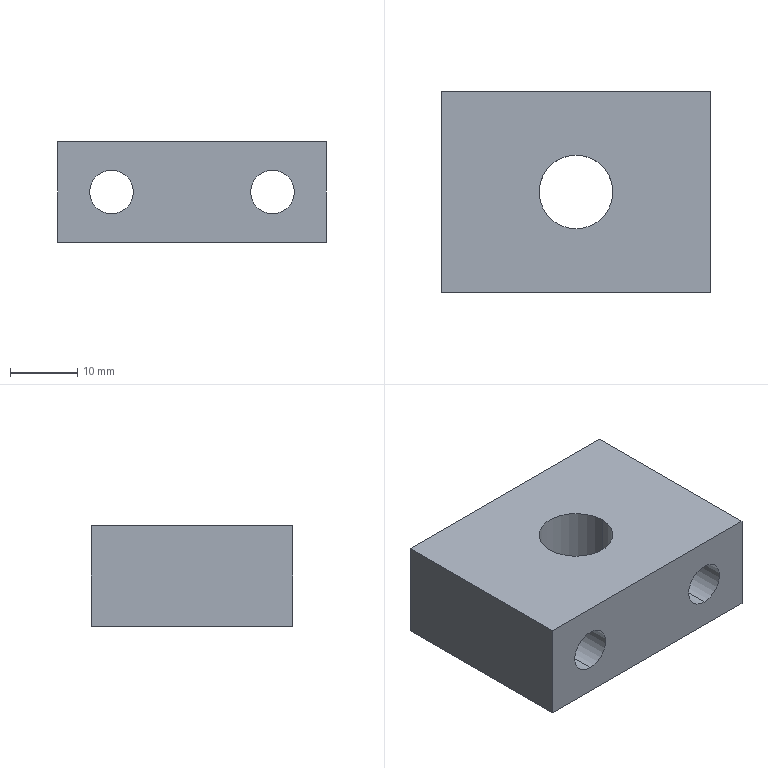Part | STEP file | 0245_206_Block | 1 solid | 12 faces | box 40 x 30 x 15 mm | volume 14584 mm3 | cylinder 6 | plane 6 | commonest cylinder face diameters 6.5 x4 11 x2
STEP:
#1=CARTESIAN_POINT('',(0.,0.,0.));
#2=DIRECTION('',(0.,0.,1.));
#3=DIRECTION('',(1.,0.,0.));
#4=AXIS2_PLACEMENT_3D('',#1,#2,#3);
#5=CARTESIAN_POINT('',(5.5,15.,-15.));
#6=VERTEX_POINT('',#5);
#7=CARTESIAN_POINT('',(5.5,15.,0.));
#8=VERTEX_POINT('',#7);
#9=CARTESIAN_POINT('',(5.5,15.,0.));
#10=DIRECTION('',(0.,0.,1.));
#11=VECTOR('',#10,1.);
#12=LINE('',#9,#11);
#13=CARTESIAN_POINT('',(0.,15.,0.));
#14=DIRECTION('',(0.,0.,1.));
#15=DIRECTION('',(1.,0.,0.));
#16=AXIS2_PLACEMENT_3D('',#13,#14,#15);
#17=CYLINDRICAL_SURFACE('',#16,5.5);
#18=CARTESIAN_POINT('',(6.283,0.));
#19=DIRECTION('',(0.,1.));
#20=VECTOR('',#19,1.);
#21=LINE('',#18,#20);
#22=(GEOMETRIC_REPRESENTATION_CONTEXT(2)PARAMETRIC_REPRESENTATION_CONTEXT()REPRESENTATION_CONTEXT('',''));
#23=DEFINITIONAL_REPRESENTATION('',(#21),#22);
#24=PCURVE('',#17,#23);
#25=CARTESIAN_POINT('',(0.,15.,0.));
#26=DIRECTION('',(0.,0.,1.));
#27=DIRECTION('',(1.,0.,0.));
#28=AXIS2_PLACEMENT_3D('',#25,#26,#27);
#29=CYLINDRICAL_SURFACE('',#28,5.5);
#30=CARTESIAN_POINT('',(0.,0.));
#31=DIRECTION('',(0.,1.));
#32=VECTOR('',#31,1.);
#33=LINE('',#30,#32);
#34=(GEOMETRIC_REPRESENTATION_CONTEXT(2)PARAMETRIC_REPRESENTATION_CONTEXT()REPRESENTATION_CONTEXT('',''));
#35=DEFINITIONAL_REPRESENTATION('',(#33),#34);
#36=PCURVE('',#29,#35);
#37=SURFACE_CURVE('',#12,(#24,#36),.PCURVE_S1.);
#38=EDGE_CURVE('',#6,#8,#37,.T.);
#39=ORIENTED_EDGE('',*,*,#38,.T.);
#40=CARTESIAN_POINT('',(-5.5,15.,0.));
#41=VERTEX_POINT('',#40);
#42=CARTESIAN_POINT('',(0.,15.,0.));
#43=DIRECTION('',(0.,0.,1.));
#44=DIRECTION('',(1.,0.,0.));
#45=AXIS2_PLACEMENT_3D('',#42,#43,#44);
#46=CIRCLE('',#45,5.5);
#47=CARTESIAN_POINT('',(0.,0.));
#48=DIRECTION('',(1.,0.));
#49=VECTOR('',#48,1.);
#50=LINE('',#47,#49);
#51=(GEOMETRIC_REPRESENTATION_CONTEXT(2)PARAMETRIC_REPRESENTATION_CONTEXT()REPRESENTATION_CONTEXT('',''));
#52=DEFINITIONAL_REPRESENTATION('',(#50),#51);
#53=PCURVE('',#17,#52);
#54=CARTESIAN_POINT('',(-20.,30.,0.));
#55=DIRECTION('',(0.,0.,-1.));
#56=DIRECTION('',(-1.,0.,0.));
#57=AXIS2_PLACEMENT_3D('',#54,#55,#56);
#58=PLANE('',#57);
#59=CARTESIAN_POINT('',(-25.5,-15.));
#60=CARTESIAN_POINT('',(-25.5,-5.474));
#61=CARTESIAN_POINT('',(-17.25,-10.237));
#62=CARTESIAN_POINT('',(-9.,-15.));
#63=CARTESIAN_POINT('',(-17.25,-19.763));
#64=CARTESIAN_POINT('',(-25.5,-24.526));
#65=CARTESIAN_POINT('',(-25.5,-15.));
#66=(BOUNDED_CURVE()B_SPLINE_CURVE(2,(#59,#60,#61,#62,#63,#64,#65),.UNSPECIFIED.,.T.,.F.)B_SPLINE_CURVE_WITH_KNOTS((1,2,2,2,2,1),(-2.094,0.,2.094,4.189,6.283,8.378),.UNSPECIFIED.)CURVE()GEOMETRIC_REPRESENTATION_ITEM()RATIONAL_B_SPLINE_CURVE((1.,0.5,1.,0.5,1.,0.5,1.))REPRESENTATION_ITEM(''));
#67=(GEOMETRIC_REPRESENTATION_CONTEXT(2)PARAMETRIC_REPRESENTATION_CONTEXT()REPRESENTATION_CONTEXT('',''));
#68=DEFINITIONAL_REPRESENTATION('',(#66),#67);
#69=PCURVE('',#58,#68);
#70=SURFACE_CURVE('',#46,(#53,#69),.PCURVE_S1.);
#71=EDGE_CURVE('',#41,#8,#70,.T.);
#72=ORIENTED_EDGE('',*,*,#71,.F.);
#73=CARTESIAN_POINT('',(-5.5,15.,-15.));
#74=VERTEX_POINT('',#73);
#75=CARTESIAN_POINT('',(-5.5,15.,0.));
#76=DIRECTION('',(0.,0.,1.));
#77=VECTOR('',#76,1.);
#78=LINE('',#75,#77);
#79=CARTESIAN_POINT('',(3.142,0.));
#80=DIRECTION('',(0.,1.));
#81=VECTOR('',#80,1.);
#82=LINE('',#79,#81);
#83=(GEOMETRIC_REPRESENTATION_CONTEXT(2)PARAMETRIC_REPRESENTATION_CONTEXT()REPRESENTATION_CONTEXT('',''));
#84=DEFINITIONAL_REPRESENTATION('',(#82),#83);
#85=PCURVE('',#17,#84);
#86=CARTESIAN_POINT('',(3.142,0.));
#87=DIRECTION('',(0.,1.));
#88=VECTOR('',#87,1.);
#89=LINE('',#86,#88);
#90=(GEOMETRIC_REPRESENTATION_CONTEXT(2)PARAMETRIC_REPRESENTATION_CONTEXT()REPRESENTATION_CONTEXT('',''));
#91=DEFINITIONAL_REPRESENTATION('',(#89),#90);
#92=PCURVE('',#29,#91);
#93=SURFACE_CURVE('',#78,(#85,#92),.PCURVE_S1.);
#94=EDGE_CURVE('',#74,#41,#93,.T.);
#95=ORIENTED_EDGE('',*,*,#94,.F.);
#96=CARTESIAN_POINT('',(0.,15.,-15.));
#97=DIRECTION('',(0.,0.,1.));
#98=DIRECTION('',(1.,0.,0.));
#99=AXIS2_PLACEMENT_3D('',#96,#97,#98);
#100=CIRCLE('',#99,5.5);
#101=CARTESIAN_POINT('',(0.,-15.));
#102=DIRECTION('',(1.,0.));
#103=VECTOR('',#102,1.);
#104=LINE('',#101,#103);
#105=(GEOMETRIC_REPRESENTATION_CONTEXT(2)PARAMETRIC_REPRESENTATION_CONTEXT()REPRESENTATION_CONTEXT('',''));
#106=DEFINITIONAL_REPRESENTATION('',(#104),#105);
#107=PCURVE('',#17,#106);
#108=CARTESIAN_POINT('',(-20.,30.,-15.));
#109=DIRECTION('',(0.,0.,-1.));
#110=DIRECTION('',(-1.,0.,0.));
#111=AXIS2_PLACEMENT_3D('',#108,#109,#110);
#112=PLANE('',#111);
#113=CARTESIAN_POINT('',(-25.5,-15.));
#114=CARTESIAN_POINT('',(-25.5,-5.474));
#115=CARTESIAN_POINT('',(-17.25,-10.237));
#116=CARTESIAN_POINT('',(-9.,-15.));
#117=CARTESIAN_POINT('',(-17.25,-19.763));
#118=CARTESIAN_POINT('',(-25.5,-24.526));
#119=CARTESIAN_POINT('',(-25.5,-15.));
#120=(BOUNDED_CURVE()B_SPLINE_CURVE(2,(#113,#114,#115,#116,#117,#118,#119),.UNSPECIFIED.,.T.,.F.)B_SPLINE_CURVE_WITH_KNOTS((1,2,2,2,2,1),(-2.094,0.,2.094,4.189,6.283,8.378),.UNSPECIFIED.)CURVE()GEOMETRIC_REPRESENTATION_ITEM()RATIONAL_B_SPLINE_CURVE((1.,0.5,1.,0.5,1.,0.5,1.))REPRESENTATION_ITEM(''));
#121=(GEOMETRIC_REPRESENTATION_CONTEXT(2)PARAMETRIC_REPRESENTATION_CONTEXT()REPRESENTATION_CONTEXT('',''));
#122=DEFINITIONAL_REPRESENTATION('',(#120),#121);
#123=PCURVE('',#112,#122);
#124=SURFACE_CURVE('',#100,(#107,#123),.PCURVE_S1.);
#125=EDGE_CURVE('',#74,#6,#124,.T.);
#126=ORIENTED_EDGE('',*,*,#125,.T.);
#127=EDGE_LOOP('',(#39,#72,#95,#126));
#128=FACE_BOUND('',#127,.F.);
#129=ADVANCED_FACE('',(#128),#17,.F.);
#130=CARTESIAN_POINT('',(-12.,0.,-4.25));
#131=VERTEX_POINT('',#130);
#132=CARTESIAN_POINT('',(-12.,30.,-4.25));
#133=VERTEX_POINT('',#132);
#134=CARTESIAN_POINT('',(-12.,30.,-4.25));
#135=DIRECTION('',(0.,1.,0.));
#136=VECTOR('',#135,1.);
#137=LINE('',#134,#136);
#138=CARTESIAN_POINT('',(-12.,30.,-7.5));
#139=DIRECTION('',(0.,1.,0.));
#140=DIRECTION('',(0.,0.,1.));
#141=AXIS2_PLACEMENT_3D('',#138,#139,#140);
#142=CYLINDRICAL_SURFACE('',#141,3.25);
#143=CARTESIAN_POINT('',(6.283,0.));
#144=DIRECTION('',(0.,1.));
#145=VECTOR('',#144,1.);
#146=LINE('',#143,#145);
#147=(GEOMETRIC_REPRESENTATION_CONTEXT(2)PARAMETRIC_REPRESENTATION_CONTEXT()REPRESENTATION_CONTEXT('',''));
#148=DEFINITIONAL_REPRESENTATION('',(#146),#147);
#149=PCURVE('',#142,#148);
#150=CARTESIAN_POINT('',(-12.,30.,-7.5));
#151=DIRECTION('',(0.,1.,0.));
#152=DIRECTION('',(0.,0.,1.));
#153=AXIS2_PLACEMENT_3D('',#150,#151,#152);
#154=CYLINDRICAL_SURFACE('',#153,3.25);
#155=CARTESIAN_POINT('',(0.,0.));
#156=DIRECTION('',(0.,1.));
#157=VECTOR('',#156,1.);
#158=LINE('',#155,#157);
#159=(GEOMETRIC_REPRESENTATION_CONTEXT(2)PARAMETRIC_REPRESENTATION_CONTEXT()REPRESENTATION_CONTEXT('',''));
#160=DEFINITIONAL_REPRESENTATION('',(#158),#159);
#161=PCURVE('',#154,#160);
#162=SURFACE_CURVE('',#137,(#149,#161),.PCURVE_S1.);
#163=EDGE_CURVE('',#131,#133,#162,.T.);
#164=ORIENTED_EDGE('',*,*,#163,.T.);
#165=CARTESIAN_POINT('',(-12.,30.,-10.75));
#166=VERTEX_POINT('',#165);
#167=CARTESIAN_POINT('',(-12.,30.,-7.5));
#168=DIRECTION('',(0.,1.,0.));
#169=DIRECTION('',(0.,0.,1.));
#170=AXIS2_PLACEMENT_3D('',#167,#168,#169);
#171=CIRCLE('',#170,3.25);
#172=CARTESIAN_POINT('',(0.,0.));
#173=DIRECTION('',(1.,0.));
#174=VECTOR('',#173,1.);
#175=LINE('',#172,#174);
#176=(GEOMETRIC_REPRESENTATION_CONTEXT(2)PARAMETRIC_REPRESENTATION_CONTEXT()REPRESENTATION_CONTEXT('',''));
#177=DEFINITIONAL_REPRESENTATION('',(#175),#176);
#178=PCURVE('',#142,#177);
#179=CARTESIAN_POINT('',(-20.,30.,-15.));
#180=DIRECTION('',(0.,1.,0.));
#181=DIRECTION('',(0.,0.,1.));
#182=AXIS2_PLACEMENT_3D('',#179,#180,#181);
#183=PLANE('',#182);
#184=CARTESIAN_POINT('',(7.5,8.));
#185=DIRECTION('',(1.,0.));
#186=AXIS2_PLACEMENT_2D('',#184,#185);
#187=CIRCLE('',#186,3.25);
#188=(GEOMETRIC_REPRESENTATION_CONTEXT(2)PARAMETRIC_REPRESENTATION_CONTEXT()REPRESENTATION_CONTEXT('',''));
#189=DEFINITIONAL_REPRESENTATION('',(#187),#188);
#190=PCURVE('',#183,#189);
#191=SURFACE_CURVE('',#171,(#178,#190),.PCURVE_S1.);
#192=EDGE_CURVE('',#166,#133,#191,.T.);
#193=ORIENTED_EDGE('',*,*,#192,.F.);
#194=CARTESIAN_POINT('',(-12.,0.,-10.75));
#195=VERTEX_POINT('',#194);
#196=CARTESIAN_POINT('',(-12.,30.,-10.75));
#197=DIRECTION('',(0.,1.,0.));
#198=VECTOR('',#197,1.);
#199=LINE('',#196,#198);
#200=CARTESIAN_POINT('',(3.142,0.));
#201=DIRECTION('',(0.,1.));
#202=VECTOR('',#201,1.);
#203=LINE('',#200,#202);
#204=(GEOMETRIC_REPRESENTATION_CONTEXT(2)PARAMETRIC_REPRESENTATION_CONTEXT()REPRESENTATION_CONTEXT('',''));
#205=DEFINITIONAL_REPRESENTATION('',(#203),#204);
#206=PCURVE('',#142,#205);
#207=CARTESIAN_POINT('',(3.142,0.));
#208=DIRECTION('',(0.,1.));
#209=VECTOR('',#208,1.);
#210=LINE('',#207,#209);
#211=(GEOMETRIC_REPRESENTATION_CONTEXT(2)PARAMETRIC_REPRESENTATION_CONTEXT()REPRESENTATION_CONTEXT('',''));
#212=DEFINITIONAL_REPRESENTATION('',(#210),#211);
#213=PCURVE('',#154,#212);
#214=SURFACE_CURVE('',#199,(#206,#213),.PCURVE_S1.);
#215=EDGE_CURVE('',#195,#166,#214,.T.);
#216=ORIENTED_EDGE('',*,*,#215,.F.);
#217=CARTESIAN_POINT('',(-12.,0.,-7.5));
#218=DIRECTION('',(0.,1.,0.));
#219=DIRECTION('',(0.,0.,1.));
#220=AXIS2_PLACEMENT_3D('',#217,#218,#219);
#221=CIRCLE('',#220,3.25);
#222=CARTESIAN_POINT('',(0.,-30.));
#223=DIRECTION('',(1.,0.));
#224=VECTOR('',#223,1.);
#225=LINE('',#222,#224);
#226=(GEOMETRIC_REPRESENTATION_CONTEXT(2)PARAMETRIC_REPRESENTATION_CONTEXT()REPRESENTATION_CONTEXT('',''));
#227=DEFINITIONAL_REPRESENTATION('',(#225),#226);
#228=PCURVE('',#142,#227);
#229=CARTESIAN_POINT('',(-20.,0.,-15.));
#230=DIRECTION('',(0.,-1.,0.));
#231=DIRECTION('',(0.,0.,-1.));
#232=AXIS2_PLACEMENT_3D('',#229,#230,#231);
#233=PLANE('',#232);
#234=CARTESIAN_POINT('',(-10.75,8.));
#235=CARTESIAN_POINT('',(-10.75,13.629));
#236=CARTESIAN_POINT('',(-5.875,10.815));
#237=CARTESIAN_POINT('',(-1.,8.));
#238=CARTESIAN_POINT('',(-5.875,5.185));
#239=CARTESIAN_POINT('',(-10.75,2.371));
#240=CARTESIAN_POINT('',(-10.75,8.));
#241=(BOUNDED_CURVE()B_SPLINE_CURVE(2,(#234,#235,#236,#237,#238,#239,#240),.UNSPECIFIED.,.T.,.F.)B_SPLINE_CURVE_WITH_KNOTS((1,2,2,2,2,1),(-2.094,0.,2.094,4.189,6.283,8.378),.UNSPECIFIED.)CURVE()GEOMETRIC_REPRESENTATION_ITEM()RATIONAL_B_SPLINE_CURVE((1.,0.5,1.,0.5,1.,0.5,1.))REPRESENTATION_ITEM(''));
#242=(GEOMETRIC_REPRESENTATION_CONTEXT(2)PARAMETRIC_REPRESENTATION_CONTEXT()REPRESENTATION_CONTEXT('',''));
#243=DEFINITIONAL_REPRESENTATION('',(#241),#242);
#244=PCURVE('',#233,#243);
#245=SURFACE_CURVE('',#221,(#228,#244),.PCURVE_S1.);
#246=EDGE_CURVE('',#195,#131,#245,.T.);
#247=ORIENTED_EDGE('',*,*,#246,.T.);
#248=EDGE_LOOP('',(#164,#193,#216,#247));
#249=FACE_BOUND('',#248,.F.);
#250=ADVANCED_FACE('',(#249),#142,.F.);
#251=CARTESIAN_POINT('',(12.,0.,-4.25));
#252=VERTEX_POINT('',#251);
#253=CARTESIAN_POINT('',(12.,30.,-4.25));
#254=VERTEX_POINT('',#253);
#255=CARTESIAN_POINT('',(12.,30.,-4.25));
#256=DIRECTION('',(0.,1.,0.));
#257=VECTOR('',#256,1.);
#258=LINE('',#255,#257);
#259=CARTESIAN_POINT('',(12.,30.,-7.5));
#260=DIRECTION('',(0.,1.,0.));
#261=DIRECTION('',(0.,0.,1.));
#262=AXIS2_PLACEMENT_3D('',#259,#260,#261);
#263=CYLINDRICAL_SURFACE('',#262,3.25);
#264=CARTESIAN_POINT('',(6.283,0.));
#265=DIRECTION('',(0.,1.));
#266=VECTOR('',#265,1.);
#267=LINE('',#264,#266);
#268=(GEOMETRIC_REPRESENTATION_CONTEXT(2)PARAMETRIC_REPRESENTATION_CONTEXT()REPRESENTATION_CONTEXT('',''));
#269=DEFINITIONAL_REPRESENTATION('',(#267),#268);
#270=PCURVE('',#263,#269);
#271=CARTESIAN_POINT('',(12.,30.,-7.5));
#272=DIRECTION('',(0.,1.,0.));
#273=DIRECTION('',(0.,0.,1.));
#274=AXIS2_PLACEMENT_3D('',#271,#272,#273);
#275=CYLINDRICAL_SURFACE('',#274,3.25);
#276=CARTESIAN_POINT('',(0.,0.));
#277=DIRECTION('',(0.,1.));
#278=VECTOR('',#277,1.);
#279=LINE('',#276,#278);
#280=(GEOMETRIC_REPRESENTATION_CONTEXT(2)PARAMETRIC_REPRESENTATION_CONTEXT()REPRESENTATION_CONTEXT('',''));
#281=DEFINITIONAL_REPRESENTATION('',(#279),#280);
#282=PCURVE('',#275,#281);
#283=SURFACE_CURVE('',#258,(#270,#282),.PCURVE_S1.);
#284=EDGE_CURVE('',#252,#254,#283,.T.);
#285=ORIENTED_EDGE('',*,*,#284,.T.);
#286=CARTESIAN_POINT('',(12.,30.,-10.75));
#287=VERTEX_POINT('',#286);
#288=CARTESIAN_POINT('',(12.,30.,-7.5));
#289=DIRECTION('',(0.,1.,0.));
#290=DIRECTION('',(0.,0.,1.));
#291=AXIS2_PLACEMENT_3D('',#288,#289,#290);
#292=CIRCLE('',#291,3.25);
#293=CARTESIAN_POINT('',(0.,0.));
#294=DIRECTION('',(1.,0.));
#295=VECTOR('',#294,1.);
#296=LINE('',#293,#295);
#297=(GEOMETRIC_REPRESENTATION_CONTEXT(2)PARAMETRIC_REPRESENTATION_CONTEXT()REPRESENTATION_CONTEXT('',''));
#298=DEFINITIONAL_REPRESENTATION('',(#296),#297);
#299=PCURVE('',#263,#298);
#300=CARTESIAN_POINT('',(7.5,32.));
#301=DIRECTION('',(1.,0.));
#302=AXIS2_PLACEMENT_2D('',#300,#301);
#303=CIRCLE('',#302,3.25);
#304=(GEOMETRIC_REPRESENTATION_CONTEXT(2)PARAMETRIC_REPRESENTATION_CONTEXT()REPRESENTATION_CONTEXT('',''));
#305=DEFINITIONAL_REPRESENTATION('',(#303),#304);
#306=PCURVE('',#183,#305);
#307=SURFACE_CURVE('',#292,(#299,#306),.PCURVE_S1.);
#308=EDGE_CURVE('',#287,#254,#307,.T.);
#309=ORIENTED_EDGE('',*,*,#308,.F.);
#310=CARTESIAN_POINT('',(12.,0.,-10.75));
#311=VERTEX_POINT('',#310);
#312=CARTESIAN_POINT('',(12.,30.,-10.75));
#313=DIRECTION('',(0.,1.,0.));
#314=VECTOR('',#313,1.);
#315=LINE('',#312,#314);
#316=CARTESIAN_POINT('',(3.142,0.));
#317=DIRECTION('',(0.,1.));
#318=VECTOR('',#317,1.);
#319=LINE('',#316,#318);
#320=(GEOMETRIC_REPRESENTATION_CONTEXT(2)PARAMETRIC_REPRESENTATION_CONTEXT()REPRESENTATION_CONTEXT('',''));
#321=DEFINITIONAL_REPRESENTATION('',(#319),#320);
#322=PCURVE('',#263,#321);
#323=CARTESIAN_POINT('',(3.142,0.));
#324=DIRECTION('',(0.,1.));
#325=VECTOR('',#324,1.);
#326=LINE('',#323,#325);
#327=(GEOMETRIC_REPRESENTATION_CONTEXT(2)PARAMETRIC_REPRESENTATION_CONTEXT()REPRESENTATION_CONTEXT('',''));
#328=DEFINITIONAL_REPRESENTATION('',(#326),#327);
#329=PCURVE('',#275,#328);
#330=SURFACE_CURVE('',#315,(#322,#329),.PCURVE_S1.);
#331=EDGE_CURVE('',#311,#287,#330,.T.);
#332=ORIENTED_EDGE('',*,*,#331,.F.);
#333=CARTESIAN_POINT('',(12.,0.,-7.5));
#334=DIRECTION('',(0.,1.,0.));
#335=DIRECTION('',(0.,0.,1.));
#336=AXIS2_PLACEMENT_3D('',#333,#334,#335);
#337=CIRCLE('',#336,3.25);
#338=CARTESIAN_POINT('',(0.,-30.));
#339=DIRECTION('',(1.,0.));
#340=VECTOR('',#339,1.);
#341=LINE('',#338,#340);
#342=(GEOMETRIC_REPRESENTATION_CONTEXT(2)PARAMETRIC_REPRESENTATION_CONTEXT()REPRESENTATION_CONTEXT('',''));
#343=DEFINITIONAL_REPRESENTATION('',(#341),#342);
#344=PCURVE('',#263,#343);
#345=CARTESIAN_POINT('',(-10.75,32.));
#346=CARTESIAN_POINT('',(-10.75,37.629));
#347=CARTESIAN_POINT('',(-5.875,34.815));
#348=CARTESIAN_POINT('',(-1.,32.));
#349=CARTESIAN_POINT('',(-5.875,29.185));
#350=CARTESIAN_POINT('',(-10.75,26.371));
#351=CARTESIAN_POINT('',(-10.75,32.));
#352=(BOUNDED_CURVE()B_SPLINE_CURVE(2,(#345,#346,#347,#348,#349,#350,#351),.UNSPECIFIED.,.T.,.F.)B_SPLINE_CURVE_WITH_KNOTS((1,2,2,2,2,1),(-2.094,0.,2.094,4.189,6.283,8.378),.UNSPECIFIED.)CURVE()GEOMETRIC_REPRESENTATION_ITEM()RATIONAL_B_SPLINE_CURVE((1.,0.5,1.,0.5,1.,0.5,1.))REPRESENTATION_ITEM(''));
#353=(GEOMETRIC_REPRESENTATION_CONTEXT(2)PARAMETRIC_REPRESENTATION_CONTEXT()REPRESENTATION_CONTEXT('',''));
#354=DEFINITIONAL_REPRESENTATION('',(#352),#353);
#355=PCURVE('',#233,#354);
#356=SURFACE_CURVE('',#337,(#344,#355),.PCURVE_S1.);
#357=EDGE_CURVE('',#311,#252,#356,.T.);
#358=ORIENTED_EDGE('',*,*,#357,.T.);
#359=EDGE_LOOP('',(#285,#309,#332,#358));
#360=FACE_BOUND('',#359,.F.);
#361=ADVANCED_FACE('',(#360),#263,.F.);
#362=CARTESIAN_POINT('',(-20.,30.,0.));
#363=VERTEX_POINT('',#362);
#364=CARTESIAN_POINT('',(-20.,0.,0.));
#365=VERTEX_POINT('',#364);
#366=CARTESIAN_POINT('',(-20.,0.,0.));
#367=DIRECTION('',(0.,-1.,0.));
#368=VECTOR('',#367,1.);
#369=LINE('',#366,#368);
#370=CARTESIAN_POINT('',(-20.,0.,-15.));
#371=DIRECTION('',(-1.,0.,0.));
#372=DIRECTION('',(0.,0.,1.));
#373=AXIS2_PLACEMENT_3D('',#370,#371,#372);
#374=PLANE('',#373);
#375=CARTESIAN_POINT('',(15.,0.));
#376=DIRECTION('',(0.,-1.));
#377=VECTOR('',#376,1.);
#378=LINE('',#375,#377);
#379=(GEOMETRIC_REPRESENTATION_CONTEXT(2)PARAMETRIC_REPRESENTATION_CONTEXT()REPRESENTATION_CONTEXT('',''));
#380=DEFINITIONAL_REPRESENTATION('',(#378),#379);
#381=PCURVE('',#374,#380);
#382=CARTESIAN_POINT('',(0.,-30.));
#383=DIRECTION('',(0.,-1.));
#384=VECTOR('',#383,1.);
#385=LINE('',#382,#384);
#386=(GEOMETRIC_REPRESENTATION_CONTEXT(2)PARAMETRIC_REPRESENTATION_CONTEXT()REPRESENTATION_CONTEXT('',''));
#387=DEFINITIONAL_REPRESENTATION('',(#385),#386);
#388=PCURVE('',#58,#387);
#389=SURFACE_CURVE('',#369,(#381,#388),.PCURVE_S1.);
#390=EDGE_CURVE('',#363,#365,#389,.T.);
#391=ORIENTED_EDGE('',*,*,#390,.F.);
#392=CARTESIAN_POINT('',(-20.,30.,-15.));
#393=VERTEX_POINT('',#392);
#394=CARTESIAN_POINT('',(-20.,30.,-15.));
#395=DIRECTION('',(0.,0.,1.));
#396=VECTOR('',#395,1.);
#397=LINE('',#394,#396);
#398=CARTESIAN_POINT('',(0.,30.));
#399=DIRECTION('',(1.,0.));
#400=VECTOR('',#399,1.);
#401=LINE('',#398,#400);
#402=(GEOMETRIC_REPRESENTATION_CONTEXT(2)PARAMETRIC_REPRESENTATION_CONTEXT()REPRESENTATION_CONTEXT('',''));
#403=DEFINITIONAL_REPRESENTATION('',(#401),#402);
#404=PCURVE('',#374,#403);
#405=CARTESIAN_POINT('',(0.,0.));
#406=DIRECTION('',(1.,0.));
#407=VECTOR('',#406,1.);
#408=LINE('',#405,#407);
#409=(GEOMETRIC_REPRESENTATION_CONTEXT(2)PARAMETRIC_REPRESENTATION_CONTEXT()REPRESENTATION_CONTEXT('',''));
#410=DEFINITIONAL_REPRESENTATION('',(#408),#409);
#411=PCURVE('',#183,#410);
#412=SURFACE_CURVE('',#397,(#404,#411),.PCURVE_S1.);
#413=EDGE_CURVE('',#393,#363,#412,.T.);
#414=ORIENTED_EDGE('',*,*,#413,.F.);
#415=CARTESIAN_POINT('',(-20.,0.,-15.));
#416=VERTEX_POINT('',#415);
#417=CARTESIAN_POINT('',(-20.,0.,-15.));
#418=DIRECTION('',(0.,-1.,0.));
#419=VECTOR('',#418,1.);
#420=LINE('',#417,#419);
#421=CARTESIAN_POINT('',(0.,0.));
#422=DIRECTION('',(0.,-1.));
#423=VECTOR('',#422,1.);
#424=LINE('',#421,#423);
#425=(GEOMETRIC_REPRESENTATION_CONTEXT(2)PARAMETRIC_REPRESENTATION_CONTEXT()REPRESENTATION_CONTEXT('',''));
#426=DEFINITIONAL_REPRESENTATION('',(#424),#425);
#427=PCURVE('',#374,#426);
#428=CARTESIAN_POINT('',(0.,-30.));
#429=DIRECTION('',(0.,-1.));
#430=VECTOR('',#429,1.);
#431=LINE('',#428,#430);
#432=(GEOMETRIC_REPRESENTATION_CONTEXT(2)PARAMETRIC_REPRESENTATION_CONTEXT()REPRESENTATION_CONTEXT('',''));
#433=DEFINITIONAL_REPRESENTATION('',(#431),#432);
#434=PCURVE('',#112,#433);
#435=SURFACE_CURVE('',#420,(#427,#434),.PCURVE_S1.);
#436=EDGE_CURVE('',#393,#416,#435,.T.);
#437=ORIENTED_EDGE('',*,*,#436,.T.);
#438=CARTESIAN_POINT('',(-20.,0.,-15.));
#439=DIRECTION('',(0.,0.,1.));
#440=VECTOR('',#439,1.);
#441=LINE('',#438,#440);
#442=CARTESIAN_POINT('',(0.,0.));
#443=DIRECTION('',(1.,0.));
#444=VECTOR('',#443,1.);
#445=LINE('',#442,#444);
#446=(GEOMETRIC_REPRESENTATION_CONTEXT(2)PARAMETRIC_REPRESENTATION_CONTEXT()REPRESENTATION_CONTEXT('',''));
#447=DEFINITIONAL_REPRESENTATION('',(#445),#446);
#448=PCURVE('',#374,#447);
#449=CARTESIAN_POINT('',(0.,0.));
#450=DIRECTION('',(-1.,0.));
#451=VECTOR('',#450,1.);
#452=LINE('',#449,#451);
#453=(GEOMETRIC_REPRESENTATION_CONTEXT(2)PARAMETRIC_REPRESENTATION_CONTEXT()REPRESENTATION_CONTEXT('',''));
#454=DEFINITIONAL_REPRESENTATION('',(#452),#453);
#455=PCURVE('',#233,#454);
#456=SURFACE_CURVE('',#441,(#448,#455),.PCURVE_S1.);
#457=EDGE_CURVE('',#416,#365,#456,.T.);
#458=ORIENTED_EDGE('',*,*,#457,.T.);
#459=EDGE_LOOP('',(#391,#414,#437,#458));
#460=FACE_BOUND('',#459,.T.);
#461=ADVANCED_FACE('',(#460),#374,.T.);
#462=CARTESIAN_POINT('',(-12.,30.,-7.5));
#463=DIRECTION('',(0.,1.,0.));
#464=DIRECTION('',(0.,0.,1.));
#465=AXIS2_PLACEMENT_3D('',#462,#463,#464);
#466=CIRCLE('',#465,3.25);
#467=CARTESIAN_POINT('',(7.5,8.));
#468=DIRECTION('',(1.,0.));
#469=AXIS2_PLACEMENT_2D('',#467,#468);
#470=CIRCLE('',#469,3.25);
#471=(GEOMETRIC_REPRESENTATION_CONTEXT(2)PARAMETRIC_REPRESENTATION_CONTEXT()REPRESENTATION_CONTEXT('',''));
#472=DEFINITIONAL_REPRESENTATION('',(#470),#471);
#473=PCURVE('',#183,#472);
#474=CARTESIAN_POINT('',(0.,0.));
#475=DIRECTION('',(1.,0.));
#476=VECTOR('',#475,1.);
#477=LINE('',#474,#476);
#478=(GEOMETRIC_REPRESENTATION_CONTEXT(2)PARAMETRIC_REPRESENTATION_CONTEXT()REPRESENTATION_CONTEXT('',''));
#479=DEFINITIONAL_REPRESENTATION('',(#477),#478);
#480=PCURVE('',#154,#479);
#481=SURFACE_CURVE('',#466,(#473,#480),.PCURVE_S1.);
#482=EDGE_CURVE('',#133,#166,#481,.T.);
#483=ORIENTED_EDGE('',*,*,#482,.F.);
#484=ORIENTED_EDGE('',*,*,#192,.F.);
#485=EDGE_LOOP('',(#483,#484));
#486=FACE_BOUND('',#485,.T.);
#487=CARTESIAN_POINT('',(12.,30.,-7.5));
#488=DIRECTION('',(0.,1.,0.));
#489=DIRECTION('',(0.,0.,1.));
#490=AXIS2_PLACEMENT_3D('',#487,#488,#489);
#491=CIRCLE('',#490,3.25);
#492=CARTESIAN_POINT('',(7.5,32.));
#493=DIRECTION('',(1.,0.));
#494=AXIS2_PLACEMENT_2D('',#492,#493);
#495=CIRCLE('',#494,3.25);
#496=(GEOMETRIC_REPRESENTATION_CONTEXT(2)PARAMETRIC_REPRESENTATION_CONTEXT()REPRESENTATION_CONTEXT('',''));
#497=DEFINITIONAL_REPRESENTATION('',(#495),#496);
#498=PCURVE('',#183,#497);
#499=CARTESIAN_POINT('',(0.,0.));
#500=DIRECTION('',(1.,0.));
#501=VECTOR('',#500,1.);
#502=LINE('',#499,#501);
#503=(GEOMETRIC_REPRESENTATION_CONTEXT(2)PARAMETRIC_REPRESENTATION_CONTEXT()REPRESENTATION_CONTEXT('',''));
#504=DEFINITIONAL_REPRESENTATION('',(#502),#503);
#505=PCURVE('',#275,#504);
#506=SURFACE_CURVE('',#491,(#498,#505),.PCURVE_S1.);
#507=EDGE_CURVE('',#254,#287,#506,.T.);
#508=ORIENTED_EDGE('',*,*,#507,.F.);
#509=ORIENTED_EDGE('',*,*,#308,.F.);
#510=EDGE_LOOP('',(#508,#509));
#511=FACE_BOUND('',#510,.T.);
#512=CARTESIAN_POINT('',(20.,30.,0.));
#513=VERTEX_POINT('',#512);
#514=CARTESIAN_POINT('',(-20.,30.,0.));
#515=DIRECTION('',(-1.,0.,0.));
#516=VECTOR('',#515,1.);
#517=LINE('',#514,#516);
#518=CARTESIAN_POINT('',(15.,0.));
#519=DIRECTION('',(0.,-1.));
#520=VECTOR('',#519,1.);
#521=LINE('',#518,#520);
#522=(GEOMETRIC_REPRESENTATION_CONTEXT(2)PARAMETRIC_REPRESENTATION_CONTEXT()REPRESENTATION_CONTEXT('',''));
#523=DEFINITIONAL_REPRESENTATION('',(#521),#522);
#524=PCURVE('',#183,#523);
#525=CARTESIAN_POINT('',(0.,0.));
#526=DIRECTION('',(1.,0.));
#527=VECTOR('',#526,1.);
#528=LINE('',#525,#527);
#529=(GEOMETRIC_REPRESENTATION_CONTEXT(2)PARAMETRIC_REPRESENTATION_CONTEXT()REPRESENTATION_CONTEXT('',''));
#530=DEFINITIONAL_REPRESENTATION('',(#528),#529);
#531=PCURVE('',#58,#530);
#532=SURFACE_CURVE('',#517,(#524,#531),.PCURVE_S1.);
#533=EDGE_CURVE('',#513,#363,#532,.T.);
#534=ORIENTED_EDGE('',*,*,#533,.F.);
#535=CARTESIAN_POINT('',(20.,30.,-15.));
#536=VERTEX_POINT('',#535);
#537=CARTESIAN_POINT('',(20.,30.,-15.));
#538=DIRECTION('',(0.,0.,1.));
#539=VECTOR('',#538,1.);
#540=LINE('',#537,#539);
#541=CARTESIAN_POINT('',(0.,40.));
#542=DIRECTION('',(1.,0.));
#543=VECTOR('',#542,1.);
#544=LINE('',#541,#543);
#545=(GEOMETRIC_REPRESENTATION_CONTEXT(2)PARAMETRIC_REPRESENTATION_CONTEXT()REPRESENTATION_CONTEXT('',''));
#546=DEFINITIONAL_REPRESENTATION('',(#544),#545);
#547=PCURVE('',#183,#546);
#548=CARTESIAN_POINT('',(20.,0.,-15.));
#549=DIRECTION('',(1.,0.,0.));
#550=DIRECTION('',(0.,0.,-1.));
#551=AXIS2_PLACEMENT_3D('',#548,#549,#550);
#552=PLANE('',#551);
#553=CARTESIAN_POINT('',(0.,30.));
#554=DIRECTION('',(-1.,0.));
#555=VECTOR('',#554,1.);
#556=LINE('',#553,#555);
#557=(GEOMETRIC_REPRESENTATION_CONTEXT(2)PARAMETRIC_REPRESENTATION_CONTEXT()REPRESENTATION_CONTEXT('',''));
#558=DEFINITIONAL_REPRESENTATION('',(#556),#557);
#559=PCURVE('',#552,#558);
#560=SURFACE_CURVE('',#540,(#547,#559),.PCURVE_S1.);
#561=EDGE_CURVE('',#536,#513,#560,.T.);
#562=ORIENTED_EDGE('',*,*,#561,.F.);
#563=CARTESIAN_POINT('',(-20.,30.,-15.));
#564=DIRECTION('',(-1.,0.,0.));
#565=VECTOR('',#564,1.);
#566=LINE('',#563,#565);
#567=CARTESIAN_POINT('',(0.,0.));
#568=DIRECTION('',(0.,-1.));
#569=VECTOR('',#568,1.);
#570=LINE('',#567,#569);
#571=(GEOMETRIC_REPRESENTATION_CONTEXT(2)PARAMETRIC_REPRESENTATION_CONTEXT()REPRESENTATION_CONTEXT('',''));
#572=DEFINITIONAL_REPRESENTATION('',(#570),#571);
#573=PCURVE('',#183,#572);
#574=CARTESIAN_POINT('',(0.,0.));
#575=DIRECTION('',(1.,0.));
#576=VECTOR('',#575,1.);
#577=LINE('',#574,#576);
#578=(GEOMETRIC_REPRESENTATION_CONTEXT(2)PARAMETRIC_REPRESENTATION_CONTEXT()REPRESENTATION_CONTEXT('',''));
#579=DEFINITIONAL_REPRESENTATION('',(#577),#578);
#580=PCURVE('',#112,#579);
#581=SURFACE_CURVE('',#566,(#573,#580),.PCURVE_S1.);
#582=EDGE_CURVE('',#536,#393,#581,.T.);
#583=ORIENTED_EDGE('',*,*,#582,.T.);
#584=ORIENTED_EDGE('',*,*,#413,.T.);
#585=EDGE_LOOP('',(#534,#562,#583,#584));
#586=FACE_BOUND('',#585,.T.);
#587=ADVANCED_FACE('',(#486,#511,#586),#183,.T.);
#588=CARTESIAN_POINT('',(20.,0.,0.));
#589=VERTEX_POINT('',#588);
#590=CARTESIAN_POINT('',(20.,0.,0.));
#591=DIRECTION('',(0.,1.,0.));
#592=VECTOR('',#591,1.);
#593=LINE('',#590,#592);
#594=CARTESIAN_POINT('',(-15.,0.));
#595=DIRECTION('',(0.,1.));
#596=VECTOR('',#595,1.);
#597=LINE('',#594,#596);
#598=(GEOMETRIC_REPRESENTATION_CONTEXT(2)PARAMETRIC_REPRESENTATION_CONTEXT()REPRESENTATION_CONTEXT('',''));
#599=DEFINITIONAL_REPRESENTATION('',(#597),#598);
#600=PCURVE('',#552,#599);
#601=CARTESIAN_POINT('',(-40.,-30.));
#602=DIRECTION('',(0.,1.));
#603=VECTOR('',#602,1.);
#604=LINE('',#601,#603);
#605=(GEOMETRIC_REPRESENTATION_CONTEXT(2)PARAMETRIC_REPRESENTATION_CONTEXT()REPRESENTATION_CONTEXT('',''));
#606=DEFINITIONAL_REPRESENTATION('',(#604),#605);
#607=PCURVE('',#58,#606);
#608=SURFACE_CURVE('',#593,(#600,#607),.PCURVE_S1.);
#609=EDGE_CURVE('',#589,#513,#608,.T.);
#610=ORIENTED_EDGE('',*,*,#609,.F.);
#611=CARTESIAN_POINT('',(20.,0.,-15.));
#612=VERTEX_POINT('',#611);
#613=CARTESIAN_POINT('',(20.,0.,-15.));
#614=DIRECTION('',(0.,0.,1.));
#615=VECTOR('',#614,1.);
#616=LINE('',#613,#615);
#617=CARTESIAN_POINT('',(0.,0.));
#618=DIRECTION('',(-1.,0.));
#619=VECTOR('',#618,1.);
#620=LINE('',#617,#619);
#621=(GEOMETRIC_REPRESENTATION_CONTEXT(2)PARAMETRIC_REPRESENTATION_CONTEXT()REPRESENTATION_CONTEXT('',''));
#622=DEFINITIONAL_REPRESENTATION('',(#620),#621);
#623=PCURVE('',#552,#622);
#624=CARTESIAN_POINT('',(0.,40.));
#625=DIRECTION('',(-1.,0.));
#626=VECTOR('',#625,1.);
#627=LINE('',#624,#626);
#628=(GEOMETRIC_REPRESENTATION_CONTEXT(2)PARAMETRIC_REPRESENTATION_CONTEXT()REPRESENTATION_CONTEXT('',''));
#629=DEFINITIONAL_REPRESENTATION('',(#627),#628);
#630=PCURVE('',#233,#629);
#631=SURFACE_CURVE('',#616,(#623,#630),.PCURVE_S1.);
#632=EDGE_CURVE('',#612,#589,#631,.T.);
#633=ORIENTED_EDGE('',*,*,#632,.F.);
#634=CARTESIAN_POINT('',(20.,0.,-15.));
#635=DIRECTION('',(0.,1.,0.));
#636=VECTOR('',#635,1.);
#637=LINE('',#634,#636);
#638=CARTESIAN_POINT('',(0.,0.));
#639=DIRECTION('',(0.,1.));
#640=VECTOR('',#639,1.);
#641=LINE('',#638,#640);
#642=(GEOMETRIC_REPRESENTATION_CONTEXT(2)PARAMETRIC_REPRESENTATION_CONTEXT()REPRESENTATION_CONTEXT('',''));
#643=DEFINITIONAL_REPRESENTATION('',(#641),#642);
#644=PCURVE('',#552,#643);
#645=CARTESIAN_POINT('',(-40.,-30.));
#646=DIRECTION('',(0.,1.));
#647=VECTOR('',#646,1.);
#648=LINE('',#645,#647);
#649=(GEOMETRIC_REPRESENTATION_CONTEXT(2)PARAMETRIC_REPRESENTATION_CONTEXT()REPRESENTATION_CONTEXT('',''));
#650=DEFINITIONAL_REPRESENTATION('',(#648),#649);
#651=PCURVE('',#112,#650);
#652=SURFACE_CURVE('',#637,(#644,#651),.PCURVE_S1.);
#653=EDGE_CURVE('',#612,#536,#652,.T.);
#654=ORIENTED_EDGE('',*,*,#653,.T.);
#655=ORIENTED_EDGE('',*,*,#561,.T.);
#656=EDGE_LOOP('',(#610,#633,#654,#655));
#657=FACE_BOUND('',#656,.T.);
#658=ADVANCED_FACE('',(#657),#552,.T.);
#659=CARTESIAN_POINT('',(-12.,0.,-7.5));
#660=DIRECTION('',(0.,1.,0.));
#661=DIRECTION('',(0.,0.,1.));
#662=AXIS2_PLACEMENT_3D('',#659,#660,#661);
#663=CIRCLE('',#662,3.25);
#664=CARTESIAN_POINT('',(-10.75,8.));
#665=CARTESIAN_POINT('',(-10.75,13.629));
#666=CARTESIAN_POINT('',(-5.875,10.815));
#667=CARTESIAN_POINT('',(-1.,8.));
#668=CARTESIAN_POINT('',(-5.875,5.185));
#669=CARTESIAN_POINT('',(-10.75,2.371));
#670=CARTESIAN_POINT('',(-10.75,8.));
#671=(BOUNDED_CURVE()B_SPLINE_CURVE(2,(#664,#665,#666,#667,#668,#669,#670),.UNSPECIFIED.,.T.,.F.)B_SPLINE_CURVE_WITH_KNOTS((1,2,2,2,2,1),(-2.094,0.,2.094,4.189,6.283,8.378),.UNSPECIFIED.)CURVE()GEOMETRIC_REPRESENTATION_ITEM()RATIONAL_B_SPLINE_CURVE((1.,0.5,1.,0.5,1.,0.5,1.))REPRESENTATION_ITEM(''));
#672=(GEOMETRIC_REPRESENTATION_CONTEXT(2)PARAMETRIC_REPRESENTATION_CONTEXT()REPRESENTATION_CONTEXT('',''));
#673=DEFINITIONAL_REPRESENTATION('',(#671),#672);
#674=PCURVE('',#233,#673);
#675=CARTESIAN_POINT('',(0.,-30.));
#676=DIRECTION('',(1.,0.));
#677=VECTOR('',#676,1.);
#678=LINE('',#675,#677);
#679=(GEOMETRIC_REPRESENTATION_CONTEXT(2)PARAMETRIC_REPRESENTATION_CONTEXT()REPRESENTATION_CONTEXT('',''));
#680=DEFINITIONAL_REPRESENTATION('',(#678),#679);
#681=PCURVE('',#154,#680);
#682=SURFACE_CURVE('',#663,(#674,#681),.PCURVE_S1.);
#683=EDGE_CURVE('',#131,#195,#682,.T.);
#684=ORIENTED_EDGE('',*,*,#683,.T.);
#685=ORIENTED_EDGE('',*,*,#246,.T.);
#686=EDGE_LOOP('',(#684,#685));
#687=FACE_BOUND('',#686,.T.);
#688=CARTESIAN_POINT('',(12.,0.,-7.5));
#689=DIRECTION('',(0.,1.,0.));
#690=DIRECTION('',(0.,0.,1.));
#691=AXIS2_PLACEMENT_3D('',#688,#689,#690);
#692=CIRCLE('',#691,3.25);
#693=CARTESIAN_POINT('',(-10.75,32.));
#694=CARTESIAN_POINT('',(-10.75,37.629));
#695=CARTESIAN_POINT('',(-5.875,34.815));
#696=CARTESIAN_POINT('',(-1.,32.));
#697=CARTESIAN_POINT('',(-5.875,29.185));
#698=CARTESIAN_POINT('',(-10.75,26.371));
#699=CARTESIAN_POINT('',(-10.75,32.));
#700=(BOUNDED_CURVE()B_SPLINE_CURVE(2,(#693,#694,#695,#696,#697,#698,#699),.UNSPECIFIED.,.T.,.F.)B_SPLINE_CURVE_WITH_KNOTS((1,2,2,2,2,1),(-2.094,0.,2.094,4.189,6.283,8.378),.UNSPECIFIED.)CURVE()GEOMETRIC_REPRESENTATION_ITEM()RATIONAL_B_SPLINE_CURVE((1.,0.5,1.,0.5,1.,0.5,1.))REPRESENTATION_ITEM(''));
#701=(GEOMETRIC_REPRESENTATION_CONTEXT(2)PARAMETRIC_REPRESENTATION_CONTEXT()REPRESENTATION_CONTEXT('',''));
#702=DEFINITIONAL_REPRESENTATION('',(#700),#701);
#703=PCURVE('',#233,#702);
#704=CARTESIAN_POINT('',(0.,-30.));
#705=DIRECTION('',(1.,0.));
#706=VECTOR('',#705,1.);
#707=LINE('',#704,#706);
#708=(GEOMETRIC_REPRESENTATION_CONTEXT(2)PARAMETRIC_REPRESENTATION_CONTEXT()REPRESENTATION_CONTEXT('',''));
#709=DEFINITIONAL_REPRESENTATION('',(#707),#708);
#710=PCURVE('',#275,#709);
#711=SURFACE_CURVE('',#692,(#703,#710),.PCURVE_S1.);
#712=EDGE_CURVE('',#252,#311,#711,.T.);
#713=ORIENTED_EDGE('',*,*,#712,.T.);
#714=ORIENTED_EDGE('',*,*,#357,.T.);
#715=EDGE_LOOP('',(#713,#714));
#716=FACE_BOUND('',#715,.T.);
#717=CARTESIAN_POINT('',(-20.,0.,0.));
#718=DIRECTION('',(1.,0.,0.));
#719=VECTOR('',#718,1.);
#720=LINE('',#717,#719);
#721=CARTESIAN_POINT('',(-15.,0.));
#722=DIRECTION('',(0.,1.));
#723=VECTOR('',#722,1.);
#724=LINE('',#721,#723);
#725=(GEOMETRIC_REPRESENTATION_CONTEXT(2)PARAMETRIC_REPRESENTATION_CONTEXT()REPRESENTATION_CONTEXT('',''));
#726=DEFINITIONAL_REPRESENTATION('',(#724),#725);
#727=PCURVE('',#233,#726);
#728=CARTESIAN_POINT('',(0.,-30.));
#729=DIRECTION('',(-1.,0.));
#730=VECTOR('',#729,1.);
#731=LINE('',#728,#730);
#732=(GEOMETRIC_REPRESENTATION_CONTEXT(2)PARAMETRIC_REPRESENTATION_CONTEXT()REPRESENTATION_CONTEXT('',''));
#733=DEFINITIONAL_REPRESENTATION('',(#731),#732);
#734=PCURVE('',#58,#733);
#735=SURFACE_CURVE('',#720,(#727,#734),.PCURVE_S1.);
#736=EDGE_CURVE('',#365,#589,#735,.T.);
#737=ORIENTED_EDGE('',*,*,#736,.F.);
#738=ORIENTED_EDGE('',*,*,#457,.F.);
#739=CARTESIAN_POINT('',(-20.,0.,-15.));
#740=DIRECTION('',(1.,0.,0.));
#741=VECTOR('',#740,1.);
#742=LINE('',#739,#741);
#743=CARTESIAN_POINT('',(0.,0.));
#744=DIRECTION('',(0.,1.));
#745=VECTOR('',#744,1.);
#746=LINE('',#743,#745);
#747=(GEOMETRIC_REPRESENTATION_CONTEXT(2)PARAMETRIC_REPRESENTATION_CONTEXT()REPRESENTATION_CONTEXT('',''));
#748=DEFINITIONAL_REPRESENTATION('',(#746),#747);
#749=PCURVE('',#233,#748);
#750=CARTESIAN_POINT('',(0.,-30.));
#751=DIRECTION('',(-1.,0.));
#752=VECTOR('',#751,1.);
#753=LINE('',#750,#752);
#754=(GEOMETRIC_REPRESENTATION_CONTEXT(2)PARAMETRIC_REPRESENTATION_CONTEXT()REPRESENTATION_CONTEXT('',''));
#755=DEFINITIONAL_REPRESENTATION('',(#753),#754);
#756=PCURVE('',#112,#755);
#757=SURFACE_CURVE('',#742,(#749,#756),.PCURVE_S1.);
#758=EDGE_CURVE('',#416,#612,#757,.T.);
#759=ORIENTED_EDGE('',*,*,#758,.T.);
#760=ORIENTED_EDGE('',*,*,#632,.T.);
#761=EDGE_LOOP('',(#737,#738,#759,#760));
#762=FACE_BOUND('',#761,.T.);
#763=ADVANCED_FACE('',(#687,#716,#762),#233,.T.);
#764=CARTESIAN_POINT('',(0.,15.,-15.));
#765=DIRECTION('',(0.,0.,1.));
#766=DIRECTION('',(1.,0.,0.));
#767=AXIS2_PLACEMENT_3D('',#764,#765,#766);
#768=CIRCLE('',#767,5.5);
#769=CARTESIAN_POINT('',(-25.5,-15.));
#770=CARTESIAN_POINT('',(-25.5,-5.474));
#771=CARTESIAN_POINT('',(-17.25,-10.237));
#772=CARTESIAN_POINT('',(-9.,-15.));
#773=CARTESIAN_POINT('',(-17.25,-19.763));
#774=CARTESIAN_POINT('',(-25.5,-24.526));
#775=CARTESIAN_POINT('',(-25.5,-15.));
#776=(BOUNDED_CURVE()B_SPLINE_CURVE(2,(#769,#770,#771,#772,#773,#774,#775),.UNSPECIFIED.,.T.,.F.)B_SPLINE_CURVE_WITH_KNOTS((1,2,2,2,2,1),(-2.094,0.,2.094,4.189,6.283,8.378),.UNSPECIFIED.)CURVE()GEOMETRIC_REPRESENTATION_ITEM()RATIONAL_B_SPLINE_CURVE((1.,0.5,1.,0.5,1.,0.5,1.))REPRESENTATION_ITEM(''));
#777=(GEOMETRIC_REPRESENTATION_CONTEXT(2)PARAMETRIC_REPRESENTATION_CONTEXT()REPRESENTATION_CONTEXT('',''));
#778=DEFINITIONAL_REPRESENTATION('',(#776),#777);
#779=PCURVE('',#112,#778);
#780=CARTESIAN_POINT('',(0.,-15.));
#781=DIRECTION('',(1.,0.));
#782=VECTOR('',#781,1.);
#783=LINE('',#780,#782);
#784=(GEOMETRIC_REPRESENTATION_CONTEXT(2)PARAMETRIC_REPRESENTATION_CONTEXT()REPRESENTATION_CONTEXT('',''));
#785=DEFINITIONAL_REPRESENTATION('',(#783),#784);
#786=PCURVE('',#29,#785);
#787=SURFACE_CURVE('',#768,(#779,#786),.PCURVE_S1.);
#788=EDGE_CURVE('',#6,#74,#787,.T.);
#789=ORIENTED_EDGE('',*,*,#788,.T.);
#790=ORIENTED_EDGE('',*,*,#125,.T.);
#791=EDGE_LOOP('',(#789,#790));
#792=FACE_BOUND('',#791,.T.);
#793=ORIENTED_EDGE('',*,*,#436,.F.);
#794=ORIENTED_EDGE('',*,*,#582,.F.);
#795=ORIENTED_EDGE('',*,*,#653,.F.);
#796=ORIENTED_EDGE('',*,*,#758,.F.);
#797=EDGE_LOOP('',(#793,#794,#795,#796));
#798=FACE_BOUND('',#797,.T.);
#799=ADVANCED_FACE('',(#792,#798),#112,.T.);
#800=CARTESIAN_POINT('',(0.,15.,0.));
#801=DIRECTION('',(0.,0.,1.));
#802=DIRECTION('',(1.,0.,0.));
#803=AXIS2_PLACEMENT_3D('',#800,#801,#802);
#804=CIRCLE('',#803,5.5);
#805=CARTESIAN_POINT('',(-25.5,-15.));
#806=CARTESIAN_POINT('',(-25.5,-5.474));
#807=CARTESIAN_POINT('',(-17.25,-10.237));
#808=CARTESIAN_POINT('',(-9.,-15.));
#809=CARTESIAN_POINT('',(-17.25,-19.763));
#810=CARTESIAN_POINT('',(-25.5,-24.526));
#811=CARTESIAN_POINT('',(-25.5,-15.));
#812=(BOUNDED_CURVE()B_SPLINE_CURVE(2,(#805,#806,#807,#808,#809,#810,#811),.UNSPECIFIED.,.T.,.F.)B_SPLINE_CURVE_WITH_KNOTS((1,2,2,2,2,1),(-2.094,0.,2.094,4.189,6.283,8.378),.UNSPECIFIED.)CURVE()GEOMETRIC_REPRESENTATION_ITEM()RATIONAL_B_SPLINE_CURVE((1.,0.5,1.,0.5,1.,0.5,1.))REPRESENTATION_ITEM(''));
#813=(GEOMETRIC_REPRESENTATION_CONTEXT(2)PARAMETRIC_REPRESENTATION_CONTEXT()REPRESENTATION_CONTEXT('',''));
#814=DEFINITIONAL_REPRESENTATION('',(#812),#813);
#815=PCURVE('',#58,#814);
#816=CARTESIAN_POINT('',(0.,0.));
#817=DIRECTION('',(1.,0.));
#818=VECTOR('',#817,1.);
#819=LINE('',#816,#818);
#820=(GEOMETRIC_REPRESENTATION_CONTEXT(2)PARAMETRIC_REPRESENTATION_CONTEXT()REPRESENTATION_CONTEXT('',''));
#821=DEFINITIONAL_REPRESENTATION('',(#819),#820);
#822=PCURVE('',#29,#821);
#823=SURFACE_CURVE('',#804,(#815,#822),.PCURVE_S1.);
#824=EDGE_CURVE('',#8,#41,#823,.T.);
#825=ORIENTED_EDGE('',*,*,#824,.F.);
#826=ORIENTED_EDGE('',*,*,#71,.F.);
#827=EDGE_LOOP('',(#825,#826));
#828=FACE_BOUND('',#827,.T.);
#829=ORIENTED_EDGE('',*,*,#390,.T.);
#830=ORIENTED_EDGE('',*,*,#736,.T.);
#831=ORIENTED_EDGE('',*,*,#609,.T.);
#832=ORIENTED_EDGE('',*,*,#533,.T.);
#833=EDGE_LOOP('',(#829,#830,#831,#832));
#834=FACE_BOUND('',#833,.T.);
#835=ADVANCED_FACE('',(#828,#834),#58,.F.);
#836=ORIENTED_EDGE('',*,*,#507,.F.);
#837=ORIENTED_EDGE('',*,*,#284,.F.);
#838=ORIENTED_EDGE('',*,*,#712,.T.);
#839=ORIENTED_EDGE('',*,*,#331,.T.);
#840=EDGE_LOOP('',(#836,#837,#838,#839));
#841=FACE_BOUND('',#840,.F.);
#842=ADVANCED_FACE('',(#841),#275,.F.);
#843=ORIENTED_EDGE('',*,*,#482,.F.);
#844=ORIENTED_EDGE('',*,*,#163,.F.);
#845=ORIENTED_EDGE('',*,*,#683,.T.);
#846=ORIENTED_EDGE('',*,*,#215,.T.);
#847=EDGE_LOOP('',(#843,#844,#845,#846));
#848=FACE_BOUND('',#847,.F.);
#849=ADVANCED_FACE('',(#848),#154,.F.);
#850=ORIENTED_EDGE('',*,*,#824,.F.);
#851=ORIENTED_EDGE('',*,*,#38,.F.);
#852=ORIENTED_EDGE('',*,*,#788,.T.);
#853=ORIENTED_EDGE('',*,*,#94,.T.);
#854=EDGE_LOOP('',(#850,#851,#852,#853));
#855=FACE_BOUND('',#854,.F.);
#856=ADVANCED_FACE('',(#855),#29,.F.);
#857=CLOSED_SHELL('',(#129,#250,#361,#461,#587,#658,#763,#799,#835,#842,#849,#856));
#858=MANIFOLD_SOLID_BREP('',#857);
#859=(LENGTH_UNIT()NAMED_UNIT(*)SI_UNIT(.MILLI.,.METRE.));
#860=UNCERTAINTY_MEASURE_WITH_UNIT(LENGTH_MEASURE(0.0000001),#859,'','');
#861=(NAMED_UNIT(*)PLANE_ANGLE_UNIT()SI_UNIT($,.RADIAN.));
#862=(NAMED_UNIT(*)SI_UNIT($,.STERADIAN.)SOLID_ANGLE_UNIT());
#863=(GEOMETRIC_REPRESENTATION_CONTEXT(3)GLOBAL_UNCERTAINTY_ASSIGNED_CONTEXT((#860))GLOBAL_UNIT_ASSIGNED_CONTEXT((#859,#861,#862))REPRESENTATION_CONTEXT('',''));
#864=ADVANCED_BREP_SHAPE_REPRESENTATION('',(#4,#858),#863);